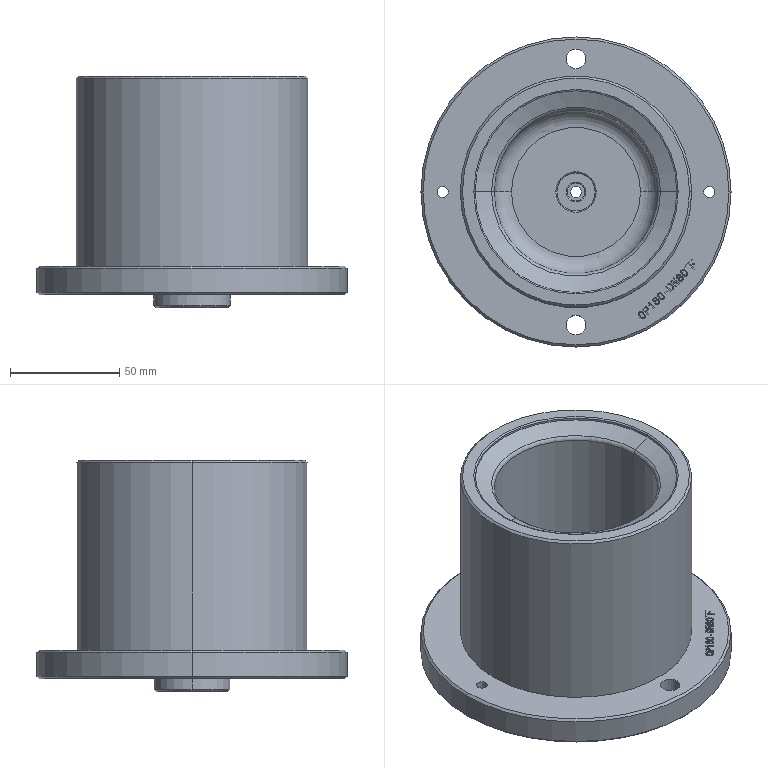Part | SolidWorks | features ICE 5, Chamfer 4, Fillet 3, HoleWzd 3, Extrusion 1, RevCut 1 | 1 solid | 184 faces | box 142 x 142 x 106 mm | volume 593458 mm3 | plane 71 | spline 69 | cylinder 24 | cone 14 | torus 6 | commonest cylinder face diameters 5 x6 9 x4 8 x2 17.5 x2 35 x2 75.1 x2